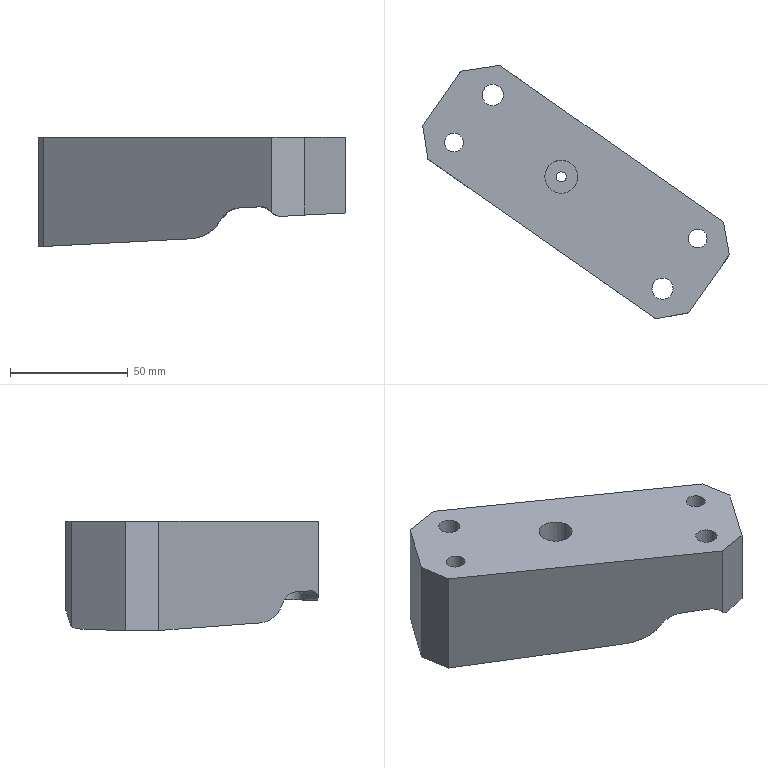Part | NX | features solid 2 | 1 solid | 39 faces | box 130.077 x 107.449 x 46.441 mm | volume 241927 mm3 | spline 15 | plane 14 | cylinder 10 | commonest cylinder face diameters 9 x4 8 x2 13 x2 4.3 x1 14 x1